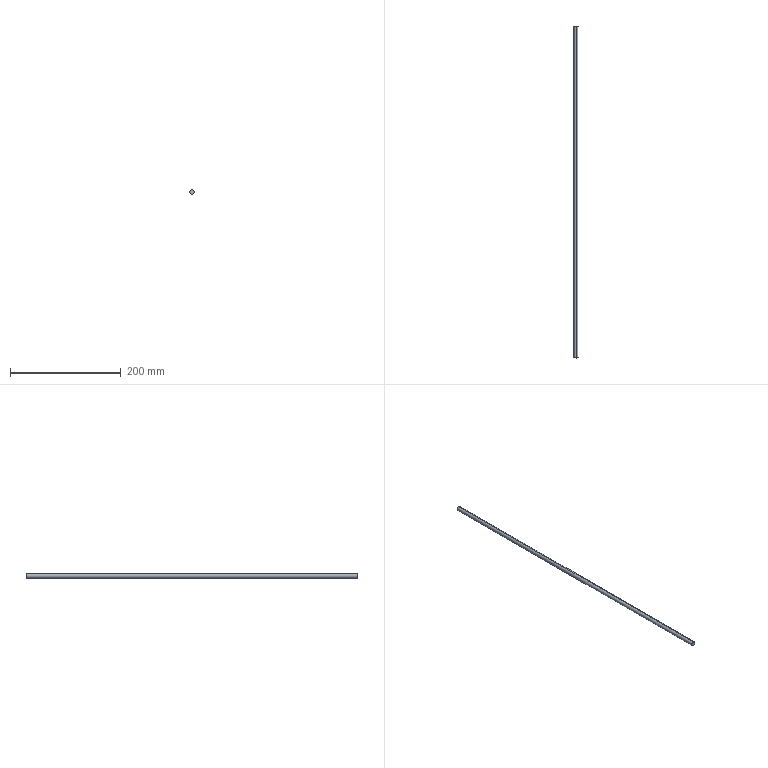Part | SolidWorks | features Extrusion 1 | 1 solid | 4 faces | box 8 x 600 x 8 mm | volume 30159 mm3 | cylinder 2 | plane 2 | commonest cylinder face diameters 8 x2
STEP:
#1=CARTESIAN_POINT('',(0.,600.,4.));
#2=VERTEX_POINT('',#1);
#3=CARTESIAN_POINT('',(0.,600.,-4.));
#4=VERTEX_POINT('',#3);
#5=CARTESIAN_POINT('',(0.,600.,0.));
#6=DIRECTION('',(0.,1.,0.));
#7=DIRECTION('',(0.,0.,1.));
#8=AXIS2_PLACEMENT_3D('',#5,#6,#7);
#9=CIRCLE('',#8,4.);
#10=EDGE_CURVE('',#2,#4,#9,.T.);
#11=ORIENTED_EDGE('',*,*,#10,.F.);
#12=CARTESIAN_POINT('',(0.,0.,4.));
#13=VERTEX_POINT('',#12);
#14=CARTESIAN_POINT('',(0.,600.,4.));
#15=DIRECTION('',(0.,-1.,0.));
#16=VECTOR('',#15,1000.);
#17=LINE('',#14,#16);
#18=EDGE_CURVE('',#2,#13,#17,.T.);
#19=ORIENTED_EDGE('',*,*,#18,.T.);
#20=CARTESIAN_POINT('',(0.,0.,-4.));
#21=VERTEX_POINT('',#20);
#22=CARTESIAN_POINT('',(0.,0.,0.));
#23=DIRECTION('',(0.,1.,0.));
#24=DIRECTION('',(0.,0.,1.));
#25=AXIS2_PLACEMENT_3D('',#22,#23,#24);
#26=CIRCLE('',#25,4.);
#27=EDGE_CURVE('',#13,#21,#26,.T.);
#28=ORIENTED_EDGE('',*,*,#27,.T.);
#29=CARTESIAN_POINT('',(0.,600.,-4.));
#30=DIRECTION('',(0.,-1.,0.));
#31=VECTOR('',#30,1000.);
#32=LINE('',#29,#31);
#33=EDGE_CURVE('',#4,#21,#32,.T.);
#34=ORIENTED_EDGE('',*,*,#33,.F.);
#35=EDGE_LOOP('',(#11,#19,#28,#34));
#36=FACE_OUTER_BOUND('',#35,.T.);
#37=CARTESIAN_POINT('',(0.,600.,0.));
#38=DIRECTION('',(0.,-1.,0.));
#39=DIRECTION('',(0.,0.,-1.));
#40=AXIS2_PLACEMENT_3D('',#37,#38,#39);
#41=CYLINDRICAL_SURFACE('',#40,4.);
#42=ADVANCED_FACE('',(#36),#41,.T.);
#43=ORIENTED_EDGE('',*,*,#18,.F.);
#44=CARTESIAN_POINT('',(0.,600.,0.));
#45=DIRECTION('',(0.,1.,0.));
#46=DIRECTION('',(0.,0.,1.));
#47=AXIS2_PLACEMENT_3D('',#44,#45,#46);
#48=CIRCLE('',#47,4.);
#49=EDGE_CURVE('',#4,#2,#48,.T.);
#50=ORIENTED_EDGE('',*,*,#49,.F.);
#51=ORIENTED_EDGE('',*,*,#33,.T.);
#52=CARTESIAN_POINT('',(0.,0.,0.));
#53=DIRECTION('',(0.,1.,0.));
#54=DIRECTION('',(0.,0.,1.));
#55=AXIS2_PLACEMENT_3D('',#52,#53,#54);
#56=CIRCLE('',#55,4.);
#57=EDGE_CURVE('',#21,#13,#56,.T.);
#58=ORIENTED_EDGE('',*,*,#57,.T.);
#59=EDGE_LOOP('',(#43,#50,#51,#58));
#60=FACE_OUTER_BOUND('',#59,.T.);
#61=CARTESIAN_POINT('',(0.,600.,0.));
#62=DIRECTION('',(0.,-1.,0.));
#63=DIRECTION('',(0.,0.,-1.));
#64=AXIS2_PLACEMENT_3D('',#61,#62,#63);
#65=CYLINDRICAL_SURFACE('',#64,4.);
#66=ADVANCED_FACE('',(#60),#65,.T.);
#67=ORIENTED_EDGE('',*,*,#49,.T.);
#68=ORIENTED_EDGE('',*,*,#10,.T.);
#69=EDGE_LOOP('',(#67,#68));
#70=FACE_OUTER_BOUND('',#69,.T.);
#71=CARTESIAN_POINT('',(0.,600.,0.));
#72=DIRECTION('',(0.,1.,0.));
#73=DIRECTION('',(0.,0.,1.));
#74=AXIS2_PLACEMENT_3D('',#71,#72,#73);
#75=PLANE('',#74);
#76=ADVANCED_FACE('',(#70),#75,.T.);
#77=ORIENTED_EDGE('',*,*,#57,.F.);
#78=ORIENTED_EDGE('',*,*,#27,.F.);
#79=EDGE_LOOP('',(#77,#78));
#80=FACE_OUTER_BOUND('',#79,.T.);
#81=CARTESIAN_POINT('',(0.,0.,0.));
#82=DIRECTION('',(0.,1.,0.));
#83=DIRECTION('',(0.,0.,1.));
#84=AXIS2_PLACEMENT_3D('',#81,#82,#83);
#85=PLANE('',#84);
#86=ADVANCED_FACE('',(#80),#85,.F.);
#87=CLOSED_SHELL('',(#42,#66,#76,#86));
#88=MANIFOLD_SOLID_BREP('',#87);
#89=CARTESIAN_POINT('',(0.,0.,0.));
#90=DIRECTION('',(0.,0.,1.));
#91=DIRECTION('',(1.,0.,0.));
#92=AXIS2_PLACEMENT_3D('',#89,#90,#91);
#93=(LENGTH_UNIT()NAMED_UNIT(*)SI_UNIT(.MILLI.,.METRE.));
#94=UNCERTAINTY_MEASURE_WITH_UNIT(LENGTH_MEASURE(0.00001),#93,'','');
#95=(NAMED_UNIT(*)PLANE_ANGLE_UNIT()SI_UNIT($,.RADIAN.));
#96=(NAMED_UNIT(*)SI_UNIT($,.STERADIAN.)SOLID_ANGLE_UNIT());
#97=(GEOMETRIC_REPRESENTATION_CONTEXT(3)GLOBAL_UNCERTAINTY_ASSIGNED_CONTEXT((#94))GLOBAL_UNIT_ASSIGNED_CONTEXT((#93,#95,#96))REPRESENTATION_CONTEXT('',''));
#98=ADVANCED_BREP_SHAPE_REPRESENTATION('',(#88,#92),#97);